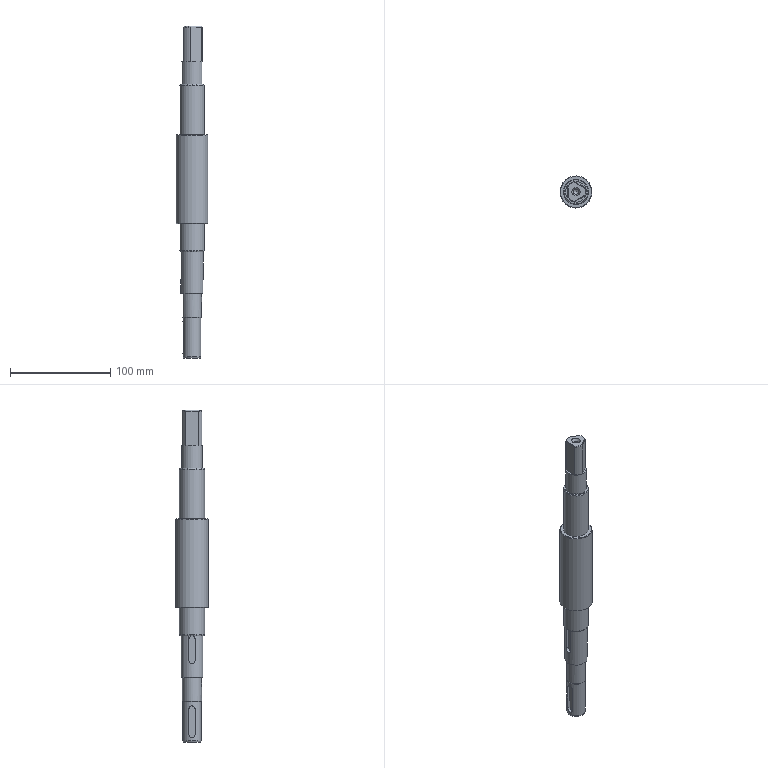NC program | NX | posted with a generic post | part box 32 x 32 x 331.3 mm
Lines 2486 to 3379 of 3379:
(PLANAR_MILL_COPY_COPY , TOOL : D6A45)
N4958 T07 M6
N4960 G54
N4962 G17 G0 G90 X-1.393 Y0.766 B0. C0. S7500 M3
N4964 G43 Z30. H7
N4966 Z0.5
N4968 G94 G1 Z-2.5 F1250.
N4970 G3 X-1.75 Y0. R1.
N4972 X-1. Y-0.75 R0.75
N4974 X-1.75 Y0. R-0.75
N4976 G1 X-2.25
N4978 G3 X-1. Y-1.25 R1.25
N4980 X-2.25 Y0. R-1.25
N4982 G1 X-2.75
N4984 G3 X-1. Y-1.75 R1.75
N4986 X-2.75 Y0. R-1.75
N4988 X-2.393 Y-0.766 R1.
N4990 G1 Z0.5
N4992 G0 Z30.
(PLANAR_MILL_COPY_COPY_COPY , TOOL : D6A45)
N4994 X-9.891
N4996 Z1.5
N4998 G1 Z-1.5
N5000 G3 X-9.534 Y0. R1.
N5002 G1 Y5.842
N5004 G2 X-9.324 Y6.455 R1.
N5006 X-2.429 Y10.436 R10.534
N5008 X-1.793 Y10.312 R1.
N5010 G1 X8.327 Y4.469
N5012 G2 X8.752 Y3.981 R1.
N5014 X8.752 Y-3.981 R10.534
N5016 X8.327 Y-4.469 R1.
N5018 G1 X-1.793 Y-10.312
N5020 G2 X-2.429 Y-10.436 R1.
N5022 X-9.324 Y-6.455 R10.534
N5024 X-9.534 Y-5.842 R1.
N5026 G1 Y0.
N5028 G3 X-9.891 Y0.766 R1.
N5030 G1 Z1.5
N5032 G0 Z30.
N5034 M5
(刀补12 , TOOL : D12)
N5036 T12 M6
N5038 G54
N5040 G17 G0 G90 X-17.318 Y-7.976 B0. C0. S5000 M3
N5042 G43 Z30. H12
N5044 Z1.
N5046 G94 G1 Z-1. F1250.
N5048 G41 X-17.224 Y-7.941 D12
N5050 X-15.65 Y-7.033
N5052 G3 X-15.05 Y-5.994 R1.2
N5054 G1 Y5.994
N5056 G2 X-13.836 Y9.635 R6.066
N5058 X-2.926 Y15.934 R16.05
N5060 X0.837 Y15.163 R6.07
N5062 G1 X11.217 Y9.17
N5064 G2 X13.763 Y6.298 R6.064
N5066 X13.794 Y-6.217 R16.033
N5068 X13.461 Y-6.9 R6.924
N5070 X11.237 Y-9.158 R5.953
N5072 G1 X0.837 Y-15.163
N5074 G2 X-2.913 Y-15.936 R6.058
N5076 X-13.843 Y-9.626 R16.05
N5078 X-15.05 Y-5.994 R6.054
N5080 G3 X-15.649 Y-4.954 R1.2
N5082 G1 X-17.45 Y-3.912
N5084 G40
N5086 X-17.544 Y-3.878
N5088 Z1.
N5090 G0 Z30.
N5092 X-17.318 Y-7.976
N5094 Z0.
N5096 G1 Z-2.
N5098 G41 X-17.224 Y-7.941
N5100 X-15.65 Y-7.033
N5102 G3 X-15.05 Y-5.994 R1.2
N5104 G1 Y6.
N5106 G2 X-13.84 Y9.63 R6.05
N5108 X-2.92 Y15.935 R16.05
N5110 X0.829 Y15.168 R6.05
N5112 G1 X11.221 Y9.168
N5114 G2 X13.76 Y6.305 R6.05
N5116 X13.76 Y-6.305 R16.05
N5118 X11.221 Y-9.168 R6.05
N5120 G1 X0.829 Y-15.168
N5122 G2 X-2.92 Y-15.935 R6.05
N5124 X-13.84 Y-9.63 R16.05
N5126 X-15.05 Y-5.994 R6.05
N5128 G3 X-15.649 Y-4.954 R1.2
N5130 G1 X-17.45 Y-3.911
N5132 G40
N5134 X-17.544 Y-3.877
N5136 Z0.
N5138 G0 Z30.
N5140 X-17.318 Y-7.976
N5142 Z-1.
N5144 G1 Z-3.
N5146 G41 X-17.224 Y-7.941
N5148 X-15.65 Y-7.033
N5150 G3 X-15.05 Y-5.994 R1.2
N5152 G1 Y6.
N5154 G2 X-13.84 Y9.63 R6.05
N5156 X-2.92 Y15.935 R16.05
N5158 X0.829 Y15.168 R6.05
N5160 G1 X11.221 Y9.168
N5162 G2 X13.76 Y6.305 R6.05
N5164 X13.76 Y-6.305 R16.05
N5166 X11.221 Y-9.168 R6.05
N5168 G1 X0.829 Y-15.168
N5170 G2 X-2.92 Y-15.935 R6.05
N5172 X-13.84 Y-9.63 R16.05
N5174 X-15.05 Y-5.994 R6.05
N5176 G3 X-15.649 Y-4.954 R1.2
N5178 G1 X-17.45 Y-3.911
N5180 G40
N5182 X-17.544 Y-3.877
N5184 Z-1.
N5186 G0 Z30.
N5188 X-17.318 Y-7.976
N5190 Z-2.
N5192 G1 Z-4.
N5194 G41 X-17.224 Y-7.941
N5196 X-15.65 Y-7.033
N5198 G3 X-15.05 Y-5.994 R1.2
N5200 G1 Y6.
N5202 G2 X-13.84 Y9.63 R6.05
N5204 X-2.92 Y15.935 R16.05
N5206 X0.829 Y15.168 R6.05
N5208 G1 X11.221 Y9.168
N5210 G2 X13.76 Y6.305 R6.05
N5212 X13.76 Y-6.305 R16.05
N5214 X11.221 Y-9.168 R6.05
N5216 G1 X0.829 Y-15.168
N5218 G2 X-2.92 Y-15.935 R6.05
N5220 X-13.84 Y-9.63 R16.05
N5222 X-15.05 Y-5.994 R6.05
N5224 G3 X-15.649 Y-4.954 R1.2
N5226 G1 X-17.45 Y-3.911
N5228 G40
N5230 X-17.544 Y-3.877
N5232 Z-2.
N5234 G0 Z30.
N5236 X-17.318 Y-7.976
N5238 Z-3.
N5240 G1 Z-5.
N5242 G41 X-17.224 Y-7.941
N5244 X-15.65 Y-7.033
N5246 G3 X-15.05 Y-5.994 R1.2
N5248 G1 Y6.
N5250 G2 X-13.84 Y9.63 R6.05
N5252 X-2.92 Y15.935 R16.05
N5254 X0.829 Y15.168 R6.05
N5256 G1 X11.221 Y9.168
N5258 G2 X13.76 Y6.305 R6.05
N5260 X13.76 Y-6.305 R16.05
N5262 X11.221 Y-9.168 R6.05
N5264 G1 X0.829 Y-15.168
N5266 G2 X-2.92 Y-15.935 R6.05
N5268 X-13.84 Y-9.63 R16.05
N5270 X-15.05 Y-5.994 R6.05
N5272 G3 X-15.649 Y-4.954 R1.2
N5274 G1 X-17.45 Y-3.911
N5276 G40
N5278 X-17.544 Y-3.877
N5280 Z-3.
N5282 G0 Z30.
N5284 X-17.318 Y-7.976
N5286 Z-4.
N5288 G1 Z-6.
N5290 G41 X-17.224 Y-7.941
N5292 X-15.65 Y-7.033
N5294 G3 X-15.05 Y-5.994 R1.2
N5296 G1 Y6.
N5298 G2 X-13.84 Y9.63 R6.05
N5300 X-2.92 Y15.935 R16.05
N5302 X0.829 Y15.168 R6.05
N5304 G1 X11.221 Y9.168
N5306 G2 X13.76 Y6.305 R6.05
N5308 X13.76 Y-6.305 R16.05
N5310 X11.221 Y-9.168 R6.05
N5312 G1 X0.829 Y-15.168
N5314 G2 X-2.92 Y-15.935 R6.05
N5316 X-13.84 Y-9.63 R16.05
N5318 X-15.05 Y-5.994 R6.05
N5320 G3 X-15.649 Y-4.954 R1.2
N5322 G1 X-17.45 Y-3.911
N5324 G40
N5326 X-17.544 Y-3.877
N5328 Z-4.
N5330 G0 Z30.
N5332 X-17.318 Y-7.976
N5334 Z-5.
N5336 G1 Z-7.
N5338 G41 X-17.224 Y-7.941
N5340 X-15.65 Y-7.033
N5342 G3 X-15.05 Y-5.994 R1.2
N5344 G1 Y6.
N5346 G2 X-13.84 Y9.63 R6.05
N5348 X-2.92 Y15.935 R16.05
N5350 X0.829 Y15.168 R6.05
N5352 G1 X11.221 Y9.168
N5354 G2 X13.76 Y6.305 R6.05
N5356 X13.76 Y-6.305 R16.05
N5358 X11.221 Y-9.168 R6.05
N5360 G1 X0.829 Y-15.168
N5362 G2 X-2.92 Y-15.935 R6.05
N5364 X-13.84 Y-9.63 R16.05
N5366 X-15.05 Y-5.994 R6.05
N5368 G3 X-15.649 Y-4.954 R1.2
N5370 G1 X-17.45 Y-3.911
N5372 G40
N5374 X-17.544 Y-3.877
N5376 Z-5.
N5378 G0 Z30.
N5380 X-17.318 Y-7.976
N5382 Z-6.
N5384 G1 Z-8.
N5386 G41 X-17.224 Y-7.941
N5388 X-15.65 Y-7.033
N5390 G3 X-15.05 Y-5.994 R1.2
N5392 G1 Y6.
N5394 G2 X-13.84 Y9.63 R6.05
N5396 X-2.92 Y15.935 R16.05
N5398 X0.829 Y15.168 R6.05
N5400 G1 X11.221 Y9.168
N5402 G2 X13.76 Y6.305 R6.05
N5404 X13.76 Y-6.305 R16.05
N5406 X11.221 Y-9.168 R6.05
N5408 G1 X0.829 Y-15.168
N5410 G2 X-2.92 Y-15.935 R6.05
N5412 X-13.84 Y-9.63 R16.05
N5414 X-15.05 Y-5.994 R6.05
N5416 G3 X-15.649 Y-4.954 R1.2
N5418 G1 X-17.45 Y-3.911
N5420 G40
N5422 X-17.544 Y-3.877
N5424 Z-6.
N5426 G0 Z30.
N5428 X-17.318 Y-7.976
N5430 Z-7.
N5432 G1 Z-9.
N5434 G41 X-17.224 Y-7.941
N5436 X-15.65 Y-7.033
N5438 G3 X-15.05 Y-5.994 R1.2
N5440 G1 Y6.
N5442 G2 X-13.84 Y9.63 R6.05
N5444 X-2.92 Y15.935 R16.05
N5446 X0.829 Y15.168 R6.05
N5448 G1 X11.221 Y9.168
N5450 G2 X13.76 Y6.305 R6.05
N5452 X13.76 Y-6.305 R16.05
N5454 X11.221 Y-9.168 R6.05
N5456 G1 X0.829 Y-15.168
N5458 G2 X-2.92 Y-15.935 R6.05
N5460 X-13.84 Y-9.63 R16.05
N5462 X-15.05 Y-5.994 R6.05
N5464 G3 X-15.649 Y-4.954 R1.2
N5466 G1 X-17.45 Y-3.911
N5468 G40
N5470 X-17.544 Y-3.877
N5472 Z-7.
N5474 G0 Z30.
N5476 X-17.318 Y-7.976
N5478 Z-8.
N5480 G1 Z-10.
N5482 G41 X-17.224 Y-7.941
N5484 X-15.65 Y-7.033
N5486 G3 X-15.05 Y-5.994 R1.2
N5488 G1 Y6.
N5490 G2 X-13.84 Y9.63 R6.05
N5492 X-2.92 Y15.935 R16.05
N5494 X0.829 Y15.168 R6.05
N5496 G1 X11.221 Y9.168
N5498 G2 X13.76 Y6.305 R6.05
N5500 X13.76 Y-6.305 R16.05
N5502 X11.221 Y-9.168 R6.05
N5504 G1 X0.829 Y-15.168
N5506 G2 X-2.92 Y-15.935 R6.05
N5508 X-13.84 Y-9.63 R16.05
N5510 X-15.05 Y-5.994 R6.05
N5512 G3 X-15.649 Y-4.954 R1.2
N5514 G1 X-17.45 Y-3.911
N5516 G40
N5518 X-17.544 Y-3.877
N5520 Z-8.
N5522 G0 Z30.
N5524 X-17.318 Y-7.976
N5526 Z-9.
N5528 G1 Z-11.
N5530 G41 X-17.224 Y-7.941
N5532 X-15.65 Y-7.033
N5534 G3 X-15.05 Y-5.994 R1.2
N5536 G1 Y6.
N5538 G2 X-13.84 Y9.63 R6.05
N5540 X-2.92 Y15.935 R16.05
N5542 X0.829 Y15.168 R6.05
N5544 G1 X11.221 Y9.168
N5546 G2 X13.76 Y6.305 R6.05
N5548 X13.76 Y-6.305 R16.05
N5550 X11.221 Y-9.168 R6.05
N5552 G1 X0.829 Y-15.168
N5554 G2 X-2.92 Y-15.935 R6.05
N5556 X-13.84 Y-9.63 R16.05
N5558 X-15.05 Y-5.994 R6.05
N5560 G3 X-15.649 Y-4.954 R1.2
N5562 G1 X-17.45 Y-3.911
N5564 G40
N5566 X-17.544 Y-3.877
N5568 Z-9.
N5570 G0 Z30.
N5572 X-17.318 Y-7.976
N5574 Z-10.
N5576 G1 Z-12.
N5578 G41 X-17.224 Y-7.941
N5580 X-15.65 Y-7.033
N5582 G3 X-15.05 Y-5.994 R1.2
N5584 G1 Y6.
N5586 G2 X-13.84 Y9.63 R6.05
N5588 X-2.92 Y15.935 R16.05
N5590 X0.829 Y15.168 R6.05
N5592 G1 X11.221 Y9.168
N5594 G2 X13.76 Y6.305 R6.05
N5596 X13.76 Y-6.305 R16.05
N5598 X11.221 Y-9.168 R6.05
N5600 G1 X0.829 Y-15.168
N5602 G2 X-2.92 Y-15.935 R6.05
N5604 X-13.84 Y-9.63 R16.05
N5606 X-15.05 Y-5.994 R6.05
N5608 G3 X-15.649 Y-4.954 R1.2
N5610 G1 X-17.45 Y-3.911
N5612 G40
N5614 X-17.544 Y-3.877
N5616 Z-10.
N5618 G0 Z30.
N5620 X-17.318 Y-7.976
N5622 Z-11.
N5624 G1 Z-13.
N5626 G41 X-17.224 Y-7.941
N5628 X-15.65 Y-7.033
N5630 G3 X-15.05 Y-5.994 R1.2
N5632 G1 Y6.
N5634 G2 X-13.84 Y9.63 R6.05
N5636 X-2.92 Y15.935 R16.05
N5638 X0.829 Y15.168 R6.05
N5640 G1 X11.221 Y9.168
N5642 G2 X13.76 Y6.305 R6.05
N5644 X13.76 Y-6.305 R16.05
N5646 X11.221 Y-9.168 R6.05
N5648 G1 X0.829 Y-15.168
N5650 G2 X-2.92 Y-15.935 R6.05
N5652 X-13.84 Y-9.63 R16.05
N5654 X-15.05 Y-5.994 R6.05
N5656 G3 X-15.649 Y-4.954 R1.2
N5658 G1 X-17.45 Y-3.911
N5660 G40
N5662 X-17.544 Y-3.877
N5664 Z-11.
N5666 G0 Z30.
N5668 X-17.318 Y-7.976
N5670 Z-12.
N5672 G1 Z-14.
N5674 G41 X-17.224 Y-7.941
N5676 X-15.65 Y-7.033
N5678 G3 X-15.05 Y-5.994 R1.2
N5680 G1 Y6.
N5682 G2 X-13.84 Y9.63 R6.05
N5684 X-2.92 Y15.935 R16.05
N5686 X0.829 Y15.168 R6.05
N5688 G1 X11.221 Y9.168
N5690 G2 X13.76 Y6.305 R6.05
N5692 X13.76 Y-6.305 R16.05
N5694 X11.221 Y-9.168 R6.05
N5696 G1 X0.829 Y-15.168
N5698 G2 X-2.92 Y-15.935 R6.05
N5700 X-13.84 Y-9.63 R16.05
N5702 X-15.05 Y-5.994 R6.05
N5704 G3 X-15.649 Y-4.954 R1.2
N5706 G1 X-17.45 Y-3.911
N5708 G40
N5710 X-17.544 Y-3.877
N5712 Z-12.
N5714 G0 Z30.
N5716 X-17.318 Y-7.976
N5718 Z-13.
N5720 G1 Z-15.
N5722 G41 X-17.224 Y-7.941
N5724 X-15.65 Y-7.033
N5726 G3 X-15.05 Y-5.994 R1.2
N5728 G1 Y6.
N5730 G2 X-13.84 Y9.63 R6.05
N5732 X-2.92 Y15.935 R16.05
N5734 X0.829 Y15.168 R6.05
N5736 G1 X11.221 Y9.168
N5738 G2 X13.76 Y6.305 R6.05
N5740 X13.76 Y-6.305 R16.05
N5742 X11.221 Y-9.168 R6.05
N5744 G1 X0.829 Y-15.168
N5746 G2 X-2.92 Y-15.935 R6.05
N5748 X-13.84 Y-9.63 R16.05
N5750 X-15.05 Y-5.994 R6.05
N5752 G3 X-15.649 Y-4.954 R1.2
N5754 G1 X-17.45 Y-3.911
N5756 G40
N5758 X-17.544 Y-3.877
N5760 Z-13.
N5762 G0 Z30.
N5764 X-17.318 Y-7.976
N5766 Z-14.
N5768 G1 Z-16.
N5770 G41 X-17.224 Y-7.941
N5772 X-15.65 Y-7.033
N5774 G3 X-15.05 Y-5.994 R1.2
N5776 G1 Y6.
N5778 G2 X-13.84 Y9.63 R6.05
N5780 X-2.92 Y15.935 R16.05
N5782 X0.829 Y15.168 R6.05
N5784 G1 X11.221 Y9.168
N5786 G2 X13.76 Y6.305 R6.05
N5788 X13.76 Y-6.305 R16.05
N5790 X11.221 Y-9.168 R6.05
N5792 G1 X0.829 Y-15.168
N5794 G2 X-2.92 Y-15.935 R6.05
N5796 X-13.84 Y-9.63 R16.05
N5798 X-15.05 Y-5.994 R6.05
N5800 G3 X-15.649 Y-4.954 R1.2
N5802 G1 X-17.45 Y-3.911
N5804 G40
N5806 X-17.544 Y-3.877
N5808 Z-14.
N5810 G0 Z30.
N5812 X-17.318 Y-7.976
N5814 Z-15.
N5816 G1 Z-17.
N5818 G41 X-17.224 Y-7.941
N5820 X-15.65 Y-7.033
N5822 G3 X-15.05 Y-5.994 R1.2
N5824 G1 Y6.
N5826 G2 X-13.84 Y9.63 R6.05
N5828 X-2.92 Y15.935 R16.05
N5830 X0.829 Y15.168 R6.05
N5832 G1 X11.221 Y9.168
N5834 G2 X13.76 Y6.305 R6.05
N5836 X13.76 Y-6.305 R16.05
N5838 X11.221 Y-9.168 R6.05
N5840 G1 X0.829 Y-15.168
N5842 G2 X-2.92 Y-15.935 R6.05
N5844 X-13.84 Y-9.63 R16.05
N5846 X-15.05 Y-5.994 R6.05
N5848 G3 X-15.649 Y-4.954 R1.2
N5850 G1 X-17.45 Y-3.911
N5852 G40
N5854 X-17.544 Y-3.877
N5856 Z-15.
N5858 G0 Z30.
N5860 X-17.318 Y-7.976
N5862 Z-16.
N5864 G1 Z-18.
N5866 G41 X-17.224 Y-7.941
N5868 X-15.65 Y-7.033
N5870 G3 X-15.05 Y-5.994 R1.2
N5872 G1 Y6.
N5874 G2 X-13.84 Y9.63 R6.05
N5876 X-2.92 Y15.935 R16.05
N5878 X0.829 Y15.168 R6.05
N5880 G1 X11.221 Y9.168
N5882 G2 X13.76 Y6.305 R6.05
N5884 X13.76 Y-6.305 R16.05
N5886 X11.221 Y-9.168 R6.05
N5888 G1 X0.829 Y-15.168
N5890 G2 X-2.92 Y-15.935 R6.05
N5892 X-13.84 Y-9.63 R16.05
N5894 X-15.05 Y-5.994 R6.05
N5896 G3 X-15.649 Y-4.954 R1.2
N5898 G1 X-17.45 Y-3.911
N5900 G40
N5902 X-17.544 Y-3.877
N5904 Z-16.
N5906 G0 Z30.
N5908 X-17.318 Y-7.976
N5910 Z-17.
N5912 G1 Z-19.
N5914 G41 X-17.224 Y-7.941
N5916 X-15.65 Y-7.033
N5918 G3 X-15.05 Y-5.994 R1.2
N5920 G1 Y6.
N5922 G2 X-13.84 Y9.63 R6.05
N5924 X-2.92 Y15.935 R16.05
N5926 X0.829 Y15.168 R6.05
N5928 G1 X11.221 Y9.168
N5930 G2 X13.76 Y6.305 R6.05
N5932 X13.76 Y-6.305 R16.05
N5934 X11.221 Y-9.168 R6.05
N5936 G1 X0.829 Y-15.168
N5938 G2 X-2.92 Y-15.935 R6.05
N5940 X-13.84 Y-9.63 R16.05
N5942 X-15.05 Y-5.994 R6.05
N5944 G3 X-15.649 Y-4.954 R1.2
N5946 G1 X-17.45 Y-3.911
N5948 G40
N5950 X-17.544 Y-3.877
N5952 Z-17.
N5954 G0 Z30.
N5956 X-17.318 Y-7.976
N5958 Z-18.
N5960 G1 Z-20.
N5962 G41 X-17.224 Y-7.941
N5964 X-15.65 Y-7.033
N5966 G3 X-15.05 Y-5.994 R1.2
N5968 G1 Y6.
N5970 G2 X-13.84 Y9.63 R6.05
N5972 X-2.92 Y15.935 R16.05
N5974 X0.829 Y15.168 R6.05
N5976 G1 X11.221 Y9.168
N5978 G2 X13.76 Y6.305 R6.05
N5980 X13.76 Y-6.305 R16.05
N5982 X11.221 Y-9.168 R6.05
N5984 G1 X0.829 Y-15.168
N5986 G2 X-2.92 Y-15.935 R6.05
N5988 X-13.84 Y-9.63 R16.05
N5990 X-15.05 Y-5.994 R6.05
N5992 G3 X-15.649 Y-4.954 R1.2
N5994 G1 X-17.45 Y-3.911
N5996 G40
N5998 X-17.544 Y-3.877
N6000 Z-18.
N6002 G0 Z30.
N6004 X-17.318 Y-7.976
N6006 Z-19.
N6008 G1 Z-21.
N6010 G41 X-17.224 Y-7.941
N6012 X-15.65 Y-7.033
N6014 G3 X-15.05 Y-5.994 R1.2
N6016 G1 Y6.
N6018 G2 X-13.84 Y9.63 R6.05
N6020 X-2.92 Y15.935 R16.05
N6022 X0.829 Y15.168 R6.05
N6024 G1 X11.221 Y9.168
N6026 G2 X13.76 Y6.305 R6.05
N6028 X13.76 Y-6.305 R16.05
N6030 X11.221 Y-9.168 R6.05
N6032 G1 X0.829 Y-15.168
N6034 G2 X-2.92 Y-15.935 R6.05
N6036 X-13.84 Y-9.63 R16.05
N6038 X-15.05 Y-5.994 R6.05
N6040 G3 X-15.649 Y-4.954 R1.2
N6042 G1 X-17.45 Y-3.911
N6044 G40
N6046 X-17.544 Y-3.877
N6048 Z-19.
N6050 G0 Z30.
N6052 X-17.318 Y-7.976
N6054 Z-20.
N6056 G1 Z-22.
N6058 G41 X-17.224 Y-7.941
N6060 X-15.65 Y-7.033
N6062 G3 X-15.05 Y-5.994 R1.2
N6064 G1 Y6.
N6066 G2 X-13.84 Y9.63 R6.05
N6068 X-2.92 Y15.935 R16.05
N6070 X0.829 Y15.168 R6.05
N6072 G1 X11.221 Y9.168
N6074 G2 X13.76 Y6.305 R6.05
N6076 X13.76 Y-6.305 R16.05
N6078 X11.221 Y-9.168 R6.05
N6080 G1 X0.829 Y-15.168
N6082 G2 X-2.92 Y-15.935 R6.05
N6084 X-13.84 Y-9.63 R16.05
N6086 X-15.05 Y-5.994 R6.05
N6088 G3 X-15.649 Y-4.954 R1.2
N6090 G1 X-17.45 Y-3.911
N6092 G40
N6094 X-17.544 Y-3.877
N6096 Z-20.
N6098 G0 Z30.
N6100 X-17.318 Y-7.976
N6102 Z-21.
N6104 G1 Z-23.
N6106 G41 X-17.224 Y-7.941
N6108 X-15.65 Y-7.033
N6110 G3 X-15.05 Y-5.994 R1.2
N6112 G1 Y6.
N6114 G2 X-13.84 Y9.63 R6.05
N6116 X-2.92 Y15.935 R16.05
N6118 X0.829 Y15.168 R6.05
N6120 G1 X11.221 Y9.168
N6122 G2 X13.76 Y6.305 R6.05
N6124 X13.76 Y-6.305 R16.05
N6126 X11.221 Y-9.168 R6.05
N6128 G1 X0.829 Y-15.168
N6130 G2 X-2.92 Y-15.935 R6.05
N6132 X-13.84 Y-9.63 R16.05
N6134 X-15.05 Y-5.994 R6.05
N6136 G3 X-15.649 Y-4.954 R1.2
N6138 G1 X-17.45 Y-3.911
N6140 G40
N6142 X-17.544 Y-3.877
N6144 Z-21.
N6146 G0 Z30.
N6148 X-17.318 Y-7.976
N6150 Z-22.
N6152 G1 Z-24.
N6154 G41 X-17.224 Y-7.941
N6156 X-15.65 Y-7.033
N6158 G3 X-15.05 Y-5.994 R1.2
N6160 G1 Y6.
N6162 G2 X-13.84 Y9.63 R6.05
N6164 X-2.92 Y15.935 R16.05
N6166 X0.829 Y15.168 R6.05
N6168 G1 X11.221 Y9.168
N6170 G2 X13.76 Y6.305 R6.05
N6172 X13.76 Y-6.305 R16.05
N6174 X11.221 Y-9.168 R6.05
N6176 G1 X0.829 Y-15.168
N6178 G2 X-2.92 Y-15.935 R6.05
N6180 X-13.84 Y-9.63 R16.05
N6182 X-15.05 Y-5.994 R6.05
N6184 G3 X-15.649 Y-4.954 R1.2
N6186 G1 X-17.45 Y-3.911
N6188 G40
N6190 X-17.544 Y-3.877
N6192 Z-22.
N6194 G0 Z30.
N6196 X-17.318 Y-7.976
N6198 Z-23.
N6200 G1 Z-25.
N6202 G41 X-17.224 Y-7.941
N6204 X-15.65 Y-7.033
N6206 G3 X-15.05 Y-5.994 R1.2
N6208 G1 Y6.
N6210 G2 X-13.84 Y9.63 R6.05
N6212 X-2.92 Y15.935 R16.05
N6214 X0.829 Y15.168 R6.05
N6216 G1 X11.221 Y9.168
N6218 G2 X13.76 Y6.305 R6.05
N6220 X13.76 Y-6.305 R16.05
N6222 X11.221 Y-9.168 R6.05
N6224 G1 X0.829 Y-15.168
N6226 G2 X-2.92 Y-15.935 R6.05
N6228 X-13.84 Y-9.63 R16.05
N6230 X-15.05 Y-5.994 R6.05
N6232 G3 X-15.649 Y-4.954 R1.2
N6234 G1 X-17.45 Y-3.911
N6236 G40
N6238 X-17.544 Y-3.877
N6240 Z-23.
N6242 G0 Z30.
N6244 X-17.318 Y-7.976
N6246 Z-24.
N6248 G1 Z-26.
N6250 G41 X-17.224 Y-7.941
N6252 X-15.65 Y-7.033
N6254 G3 X-15.05 Y-5.994 R1.2
N6256 G1 Y6.
N6258 G2 X-13.84 Y9.63 R6.05
N6260 X-2.92 Y15.935 R16.05
N6262 X0.829 Y15.168 R6.05
N6264 G1 X11.221 Y9.168
N6266 G2 X13.76 Y6.305 R6.05
N6268 X13.76 Y-6.305 R16.05
N6270 X11.221 Y-9.168 R6.05
N6272 G1 X0.829 Y-15.168
N6274 G2 X-2.92 Y-15.935 R6.05
N6276 X-13.84 Y-9.63 R16.05
N6278 X-15.05 Y-5.994 R6.05
N6280 G3 X-15.649 Y-4.954 R1.2
N6282 G1 X-17.45 Y-3.911
N6284 G40
N6286 X-17.544 Y-3.877
N6288 Z-24.
N6290 G0 Z30.
N6292 X-17.318 Y-7.976
N6294 Z-25.
N6296 G1 Z-27.
N6298 G41 X-17.224 Y-7.941
N6300 X-15.65 Y-7.033
N6302 G3 X-15.05 Y-5.994 R1.2
N6304 G1 Y6.
N6306 G2 X-13.84 Y9.63 R6.05
N6308 X-2.92 Y15.935 R16.05
N6310 X0.829 Y15.168 R6.05
N6312 G1 X11.221 Y9.168
N6314 G2 X13.76 Y6.305 R6.05
N6316 X13.76 Y-6.305 R16.05
N6318 X11.221 Y-9.168 R6.05
N6320 G1 X0.829 Y-15.168
N6322 G2 X-2.92 Y-15.935 R6.05
N6324 X-13.84 Y-9.63 R16.05
N6326 X-15.05 Y-5.994 R6.05
N6328 G3 X-15.649 Y-4.954 R1.2
N6330 G1 X-17.45 Y-3.911
N6332 G40
N6334 X-17.544 Y-3.877
N6336 Z-25.
N6338 G0 Z30.
N6340 X-17.318 Y-7.976
N6342 Z-26.
N6344 G1 Z-28.
N6346 G41 X-17.224 Y-7.941
N6348 X-15.65 Y-7.033
N6350 G3 X-15.05 Y-5.994 R1.2
N6352 G1 Y6.
N6354 G2 X-13.84 Y9.63 R6.05
N6356 X-2.92 Y15.935 R16.05
N6358 X0.829 Y15.168 R6.05
N6360 G1 X11.221 Y9.168
N6362 G2 X13.76 Y6.305 R6.05
N6364 X13.76 Y-6.305 R16.05
N6366 X11.221 Y-9.168 R6.05
N6368 G1 X0.829 Y-15.168
N6370 G2 X-2.92 Y-15.935 R6.05
N6372 X-13.84 Y-9.63 R16.05
N6374 X-15.05 Y-5.994 R6.05
N6376 G3 X-15.649 Y-4.954 R1.2
N6378 G1 X-17.45 Y-3.911
N6380 G40
N6382 X-17.544 Y-3.877
N6384 Z-26.
N6386 G0 Z30.
N6388 X-17.318 Y-7.976
N6390 Z-27.
N6392 G1 Z-29.
N6394 G41 X-17.224 Y-7.941
N6396 X-15.65 Y-7.033
N6398 G3 X-15.05 Y-5.994 R1.2
N6400 G1 Y6.
N6402 G2 X-13.84 Y9.63 R6.05
N6404 X-2.92 Y15.935 R16.05
N6406 X0.829 Y15.168 R6.05
N6408 G1 X11.221 Y9.168
N6410 G2 X13.76 Y6.305 R6.05
N6412 X13.76 Y-6.305 R16.05
N6414 X11.221 Y-9.168 R6.05
N6416 G1 X0.829 Y-15.168
N6418 G2 X-2.92 Y-15.935 R6.05
N6420 X-13.84 Y-9.63 R16.05
N6422 X-15.05 Y-5.994 R6.05
N6424 G3 X-15.649 Y-4.954 R1.2
N6426 G1 X-17.45 Y-3.911
N6428 G40
N6430 X-17.544 Y-3.877
N6432 Z-27.
N6434 G0 Z30.
N6436 X-17.318 Y-7.976
N6438 Z-28.
N6440 G1 Z-30.
N6442 G41 X-17.224 Y-7.941
N6444 X-15.65 Y-7.033
N6446 G3 X-15.05 Y-5.994 R1.2
N6448 G1 Y6.
N6450 G2 X-13.84 Y9.63 R6.05
N6452 X-2.92 Y15.935 R16.05
N6454 X0.829 Y15.168 R6.05
N6456 G1 X11.221 Y9.168
N6458 G2 X13.76 Y6.305 R6.05
N6460 X13.76 Y-6.305 R16.05
N6462 X11.221 Y-9.168 R6.05
N6464 G1 X0.829 Y-15.168
N6466 G2 X-2.92 Y-15.935 R6.05
N6468 X-13.84 Y-9.63 R16.05
N6470 X-15.05 Y-5.994 R6.05
N6472 G3 X-15.649 Y-4.954 R1.2
N6474 G1 X-17.45 Y-3.911
N6476 G40
N6478 X-17.544 Y-3.877
N6480 Z-28.
N6482 G0 Z30.
N6484 X-17.318 Y-7.976
N6486 Z-29.
N6488 G1 Z-31.
N6490 G41 X-17.224 Y-7.941
N6492 X-15.65 Y-7.033
N6494 G3 X-15.05 Y-5.994 R1.2
N6496 G1 Y6.
N6498 G2 X-13.84 Y9.63 R6.05
N6500 X-2.92 Y15.935 R16.05
N6502 X0.829 Y15.168 R6.05
N6504 G1 X11.221 Y9.168
N6506 G2 X13.76 Y6.305 R6.05
N6508 X13.76 Y-6.305 R16.05
N6510 X11.221 Y-9.168 R6.05
N6512 G1 X0.829 Y-15.168
N6514 G2 X-2.92 Y-15.935 R6.05
N6516 X-13.84 Y-9.63 R16.05
N6518 X-15.05 Y-5.994 R6.05
N6520 G3 X-15.649 Y-4.954 R1.2
N6522 G1 X-17.45 Y-3.911
N6524 G40
N6526 X-17.544 Y-3.877
N6528 Z-29.
N6530 G0 Z30.
N6532 X-17.318 Y-7.976
N6534 Z-30.
N6536 G1 Z-32.
N6538 G41 X-17.224 Y-7.941
N6540 X-15.65 Y-7.033
N6542 G3 X-15.05 Y-5.994 R1.2
N6544 G1 Y6.
N6546 G2 X-13.84 Y9.63 R6.05
N6548 X-2.92 Y15.935 R16.05
N6550 X0.829 Y15.168 R6.05
N6552 G1 X11.221 Y9.168
N6554 G2 X13.76 Y6.305 R6.05
N6556 X13.76 Y-6.305 R16.05
N6558 X11.221 Y-9.168 R6.05
N6560 G1 X0.829 Y-15.168
N6562 G2 X-2.92 Y-15.935 R6.05
N6564 X-13.84 Y-9.63 R16.05
N6566 X-15.05 Y-5.994 R6.05
N6568 G3 X-15.649 Y-4.954 R1.2
N6570 G1 X-17.45 Y-3.911
N6572 G40
N6574 X-17.544 Y-3.877
N6576 Z-30.
N6578 G0 Z30.
N6580 X-17.318 Y-7.976
N6582 Z-31.
N6584 G1 Z-33.
N6586 G41 X-17.224 Y-7.941
N6588 X-15.65 Y-7.033
N6590 G3 X-15.05 Y-5.994 R1.2
N6592 G1 Y6.
N6594 G2 X-13.84 Y9.63 R6.05
N6596 X-2.92 Y15.935 R16.05
N6598 X0.829 Y15.168 R6.05
N6600 G1 X11.221 Y9.168
N6602 G2 X13.76 Y6.305 R6.05
N6604 X13.76 Y-6.305 R16.05
N6606 X11.221 Y-9.168 R6.05
N6608 G1 X0.829 Y-15.168
N6610 G2 X-2.92 Y-15.935 R6.05
N6612 X-13.84 Y-9.63 R16.05
N6614 X-15.05 Y-5.994 R6.05
N6616 G3 X-15.649 Y-4.954 R1.2
N6618 G1 X-17.45 Y-3.911
N6620 G40
N6622 X-17.544 Y-3.877
N6624 Z-31.
N6626 G0 Z30.
N6628 X-17.318 Y-7.976
N6630 Z-32.
N6632 G1 Z-34.
N6634 G41 X-17.224 Y-7.941
N6636 X-15.65 Y-7.033
N6638 G3 X-15.05 Y-5.994 R1.2
N6640 G1 Y6.
N6642 G2 X-13.84 Y9.63 R6.05
N6644 X-2.92 Y15.935 R16.05
N6646 X0.829 Y15.168 R6.05
N6648 G1 X11.221 Y9.168
N6650 G2 X13.76 Y6.305 R6.05
N6652 X13.76 Y-6.305 R16.05
N6654 X11.221 Y-9.168 R6.05
N6656 G1 X0.829 Y-15.168
N6658 G2 X-2.92 Y-15.935 R6.05
N6660 X-13.84 Y-9.63 R16.05
N6662 X-15.05 Y-5.994 R6.05
N6664 G3 X-15.649 Y-4.954 R1.2
N6666 G1 X-17.45 Y-3.911
N6668 G40
N6670 X-17.544 Y-3.877
N6672 Z-32.
N6674 G0 Z30.
N6676 X-17.318 Y-7.976
N6678 Z-33.
N6680 G1 Z-35.
N6682 G41 X-17.224 Y-7.941
N6684 X-15.65 Y-7.033
N6686 G3 X-15.05 Y-5.994 R1.2
N6688 G1 Y6.
N6690 G2 X-13.84 Y9.63 R6.05
N6692 X-2.92 Y15.935 R16.05
N6694 X0.829 Y15.168 R6.05
N6696 G1 X11.221 Y9.168
N6698 G2 X13.76 Y6.305 R6.05
N6700 X13.76 Y-6.305 R16.05
N6702 X11.221 Y-9.168 R6.05
N6704 G1 X0.829 Y-15.168
N6706 G2 X-2.92 Y-15.935 R6.05
N6708 X-13.84 Y-9.63 R16.05
N6710 X-15.05 Y-5.994 R6.05
N6712 G3 X-15.649 Y-4.954 R1.2
N6714 G1 X-17.45 Y-3.911
N6716 G40
N6718 X-17.544 Y-3.877
N6720 Z-33.
N6722 G0 Z30.
N6724 M5
N6726 M2